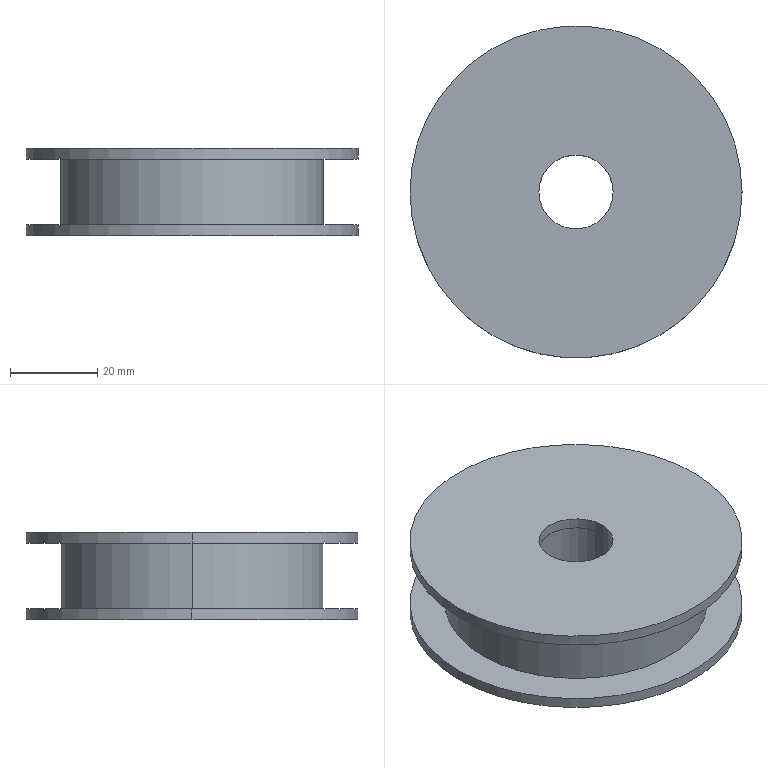Part | STEP file | WHEEL_111V11 | 3 solids | 18 faces | box 76 x 76 x 20 mm | volume 60554 mm3 | cylinder 12 | plane 6 | commonest cylinder face diameters 17 x6 76 x4 60 x2
STEP:
#1=CARTESIAN_POINT('',(0.,0.,0.));
#2=DIRECTION('',(0.,0.,1.));
#3=DIRECTION('',(1.,0.,0.));
#4=AXIS2_PLACEMENT_3D('',#1,#2,#3);
#5=CARTESIAN_POINT('',(-8.5,0.,15.));
#6=VERTEX_POINT('',#5);
#7=CARTESIAN_POINT('',(-8.5,0.,0.));
#8=VERTEX_POINT('',#7);
#9=CARTESIAN_POINT('',(-8.5,0.,15.));
#10=DIRECTION('',(0.,0.,-1.));
#11=VECTOR('',#10,1.);
#12=LINE('',#9,#11);
#13=CARTESIAN_POINT('',(0.,0.,15.));
#14=DIRECTION('',(0.,0.,-1.));
#15=DIRECTION('',(-1.,0.,0.));
#16=AXIS2_PLACEMENT_3D('',#13,#14,#15);
#17=CYLINDRICAL_SURFACE('',#16,8.5);
#18=CARTESIAN_POINT('',(6.283,0.));
#19=DIRECTION('',(0.,1.));
#20=VECTOR('',#19,1.);
#21=LINE('',#18,#20);
#22=(GEOMETRIC_REPRESENTATION_CONTEXT(2)PARAMETRIC_REPRESENTATION_CONTEXT()REPRESENTATION_CONTEXT('',''));
#23=DEFINITIONAL_REPRESENTATION('',(#21),#22);
#24=PCURVE('',#17,#23);
#25=CARTESIAN_POINT('',(0.,0.,15.));
#26=DIRECTION('',(0.,0.,-1.));
#27=DIRECTION('',(-1.,0.,0.));
#28=AXIS2_PLACEMENT_3D('',#25,#26,#27);
#29=CYLINDRICAL_SURFACE('',#28,8.5);
#30=CARTESIAN_POINT('',(0.,0.));
#31=DIRECTION('',(0.,1.));
#32=VECTOR('',#31,1.);
#33=LINE('',#30,#32);
#34=(GEOMETRIC_REPRESENTATION_CONTEXT(2)PARAMETRIC_REPRESENTATION_CONTEXT()REPRESENTATION_CONTEXT('',''));
#35=DEFINITIONAL_REPRESENTATION('',(#33),#34);
#36=PCURVE('',#29,#35);
#37=SURFACE_CURVE('',#12,(#24,#36),.PCURVE_S1.);
#38=EDGE_CURVE('',#6,#8,#37,.T.);
#39=ORIENTED_EDGE('',*,*,#38,.T.);
#40=CARTESIAN_POINT('',(8.5,0.,0.));
#41=VERTEX_POINT('',#40);
#42=CARTESIAN_POINT('',(0.,0.,0.));
#43=DIRECTION('',(0.,0.,1.));
#44=DIRECTION('',(1.,0.,0.));
#45=AXIS2_PLACEMENT_3D('',#42,#43,#44);
#46=CIRCLE('',#45,8.5);
#47=CARTESIAN_POINT('',(9.425,15.));
#48=DIRECTION('',(-1.,0.));
#49=VECTOR('',#48,1.);
#50=LINE('',#47,#49);
#51=(GEOMETRIC_REPRESENTATION_CONTEXT(2)PARAMETRIC_REPRESENTATION_CONTEXT()REPRESENTATION_CONTEXT('',''));
#52=DEFINITIONAL_REPRESENTATION('',(#50),#51);
#53=PCURVE('',#17,#52);
#54=CARTESIAN_POINT('',(0.,0.,0.));
#55=DIRECTION('',(0.,0.,1.));
#56=DIRECTION('',(1.,0.,0.));
#57=AXIS2_PLACEMENT_3D('',#54,#55,#56);
#58=PLANE('',#57);
#59=CARTESIAN_POINT('',(0.,0.));
#60=DIRECTION('',(1.,0.));
#61=AXIS2_PLACEMENT_2D('',#59,#60);
#62=CIRCLE('',#61,8.5);
#63=(GEOMETRIC_REPRESENTATION_CONTEXT(2)PARAMETRIC_REPRESENTATION_CONTEXT()REPRESENTATION_CONTEXT('',''));
#64=DEFINITIONAL_REPRESENTATION('',(#62),#63);
#65=PCURVE('',#58,#64);
#66=SURFACE_CURVE('',#46,(#53,#65),.PCURVE_S1.);
#67=EDGE_CURVE('',#8,#41,#66,.T.);
#68=ORIENTED_EDGE('',*,*,#67,.T.);
#69=CARTESIAN_POINT('',(8.5,0.,15.));
#70=VERTEX_POINT('',#69);
#71=CARTESIAN_POINT('',(8.5,0.,15.));
#72=DIRECTION('',(0.,0.,-1.));
#73=VECTOR('',#72,1.);
#74=LINE('',#71,#73);
#75=CARTESIAN_POINT('',(3.142,0.));
#76=DIRECTION('',(0.,1.));
#77=VECTOR('',#76,1.);
#78=LINE('',#75,#77);
#79=(GEOMETRIC_REPRESENTATION_CONTEXT(2)PARAMETRIC_REPRESENTATION_CONTEXT()REPRESENTATION_CONTEXT('',''));
#80=DEFINITIONAL_REPRESENTATION('',(#78),#79);
#81=PCURVE('',#17,#80);
#82=CARTESIAN_POINT('',(3.142,0.));
#83=DIRECTION('',(0.,1.));
#84=VECTOR('',#83,1.);
#85=LINE('',#82,#84);
#86=(GEOMETRIC_REPRESENTATION_CONTEXT(2)PARAMETRIC_REPRESENTATION_CONTEXT()REPRESENTATION_CONTEXT('',''));
#87=DEFINITIONAL_REPRESENTATION('',(#85),#86);
#88=PCURVE('',#29,#87);
#89=SURFACE_CURVE('',#74,(#81,#88),.PCURVE_S1.);
#90=EDGE_CURVE('',#70,#41,#89,.T.);
#91=ORIENTED_EDGE('',*,*,#90,.F.);
#92=CARTESIAN_POINT('',(0.,0.,15.));
#93=DIRECTION('',(0.,0.,1.));
#94=DIRECTION('',(1.,0.,0.));
#95=AXIS2_PLACEMENT_3D('',#92,#93,#94);
#96=CIRCLE('',#95,8.5);
#97=CARTESIAN_POINT('',(9.425,0.));
#98=DIRECTION('',(-1.,0.));
#99=VECTOR('',#98,1.);
#100=LINE('',#97,#99);
#101=(GEOMETRIC_REPRESENTATION_CONTEXT(2)PARAMETRIC_REPRESENTATION_CONTEXT()REPRESENTATION_CONTEXT('',''));
#102=DEFINITIONAL_REPRESENTATION('',(#100),#101);
#103=PCURVE('',#17,#102);
#104=CARTESIAN_POINT('',(0.,0.,15.));
#105=DIRECTION('',(0.,0.,1.));
#106=DIRECTION('',(1.,0.,0.));
#107=AXIS2_PLACEMENT_3D('',#104,#105,#106);
#108=PLANE('',#107);
#109=CARTESIAN_POINT('',(0.,0.));
#110=DIRECTION('',(1.,0.));
#111=AXIS2_PLACEMENT_2D('',#109,#110);
#112=CIRCLE('',#111,8.5);
#113=(GEOMETRIC_REPRESENTATION_CONTEXT(2)PARAMETRIC_REPRESENTATION_CONTEXT()REPRESENTATION_CONTEXT('',''));
#114=DEFINITIONAL_REPRESENTATION('',(#112),#113);
#115=PCURVE('',#108,#114);
#116=SURFACE_CURVE('',#96,(#103,#115),.PCURVE_S1.);
#117=EDGE_CURVE('',#6,#70,#116,.T.);
#118=ORIENTED_EDGE('',*,*,#117,.F.);
#119=EDGE_LOOP('',(#39,#68,#91,#118));
#120=FACE_BOUND('',#119,.F.);
#121=ADVANCED_FACE('',(#120),#17,.F.);
#122=CARTESIAN_POINT('',(30.,0.,15.));
#123=VERTEX_POINT('',#122);
#124=CARTESIAN_POINT('',(-30.,0.,15.));
#125=VERTEX_POINT('',#124);
#126=CARTESIAN_POINT('',(0.,0.,15.));
#127=DIRECTION('',(0.,0.,1.));
#128=DIRECTION('',(1.,0.,0.));
#129=AXIS2_PLACEMENT_3D('',#126,#127,#128);
#130=CIRCLE('',#129,30.);
#131=CARTESIAN_POINT('',(0.,0.,15.));
#132=DIRECTION('',(0.,0.,-1.));
#133=DIRECTION('',(-1.,0.,0.));
#134=AXIS2_PLACEMENT_3D('',#131,#132,#133);
#135=CYLINDRICAL_SURFACE('',#134,30.);
#136=CARTESIAN_POINT('',(3.142,0.));
#137=DIRECTION('',(-1.,0.));
#138=VECTOR('',#137,1.);
#139=LINE('',#136,#138);
#140=(GEOMETRIC_REPRESENTATION_CONTEXT(2)PARAMETRIC_REPRESENTATION_CONTEXT()REPRESENTATION_CONTEXT('',''));
#141=DEFINITIONAL_REPRESENTATION('',(#139),#140);
#142=PCURVE('',#135,#141);
#143=CARTESIAN_POINT('',(0.,0.));
#144=DIRECTION('',(1.,0.));
#145=AXIS2_PLACEMENT_2D('',#143,#144);
#146=CIRCLE('',#145,30.);
#147=(GEOMETRIC_REPRESENTATION_CONTEXT(2)PARAMETRIC_REPRESENTATION_CONTEXT()REPRESENTATION_CONTEXT('',''));
#148=DEFINITIONAL_REPRESENTATION('',(#146),#147);
#149=PCURVE('',#108,#148);
#150=SURFACE_CURVE('',#130,(#142,#149),.PCURVE_S1.);
#151=EDGE_CURVE('',#123,#125,#150,.T.);
#152=ORIENTED_EDGE('',*,*,#151,.F.);
#153=CARTESIAN_POINT('',(30.,0.,0.));
#154=VERTEX_POINT('',#153);
#155=CARTESIAN_POINT('',(30.,0.,15.));
#156=DIRECTION('',(0.,0.,-1.));
#157=VECTOR('',#156,1.);
#158=LINE('',#155,#157);
#159=CARTESIAN_POINT('',(3.142,0.));
#160=DIRECTION('',(0.,1.));
#161=VECTOR('',#160,1.);
#162=LINE('',#159,#161);
#163=(GEOMETRIC_REPRESENTATION_CONTEXT(2)PARAMETRIC_REPRESENTATION_CONTEXT()REPRESENTATION_CONTEXT('',''));
#164=DEFINITIONAL_REPRESENTATION('',(#162),#163);
#165=PCURVE('',#135,#164);
#166=CARTESIAN_POINT('',(0.,0.,15.));
#167=DIRECTION('',(0.,0.,-1.));
#168=DIRECTION('',(-1.,0.,0.));
#169=AXIS2_PLACEMENT_3D('',#166,#167,#168);
#170=CYLINDRICAL_SURFACE('',#169,30.);
#171=CARTESIAN_POINT('',(3.142,0.));
#172=DIRECTION('',(0.,1.));
#173=VECTOR('',#172,1.);
#174=LINE('',#171,#173);
#175=(GEOMETRIC_REPRESENTATION_CONTEXT(2)PARAMETRIC_REPRESENTATION_CONTEXT()REPRESENTATION_CONTEXT('',''));
#176=DEFINITIONAL_REPRESENTATION('',(#174),#175);
#177=PCURVE('',#170,#176);
#178=SURFACE_CURVE('',#158,(#165,#177),.PCURVE_S1.);
#179=EDGE_CURVE('',#123,#154,#178,.T.);
#180=ORIENTED_EDGE('',*,*,#179,.T.);
#181=CARTESIAN_POINT('',(-30.,0.,0.));
#182=VERTEX_POINT('',#181);
#183=CARTESIAN_POINT('',(0.,0.,0.));
#184=DIRECTION('',(0.,0.,1.));
#185=DIRECTION('',(1.,0.,0.));
#186=AXIS2_PLACEMENT_3D('',#183,#184,#185);
#187=CIRCLE('',#186,30.);
#188=CARTESIAN_POINT('',(3.142,15.));
#189=DIRECTION('',(-1.,0.));
#190=VECTOR('',#189,1.);
#191=LINE('',#188,#190);
#192=(GEOMETRIC_REPRESENTATION_CONTEXT(2)PARAMETRIC_REPRESENTATION_CONTEXT()REPRESENTATION_CONTEXT('',''));
#193=DEFINITIONAL_REPRESENTATION('',(#191),#192);
#194=PCURVE('',#135,#193);
#195=CARTESIAN_POINT('',(0.,0.));
#196=DIRECTION('',(1.,0.));
#197=AXIS2_PLACEMENT_2D('',#195,#196);
#198=CIRCLE('',#197,30.);
#199=(GEOMETRIC_REPRESENTATION_CONTEXT(2)PARAMETRIC_REPRESENTATION_CONTEXT()REPRESENTATION_CONTEXT('',''));
#200=DEFINITIONAL_REPRESENTATION('',(#198),#199);
#201=PCURVE('',#58,#200);
#202=SURFACE_CURVE('',#187,(#194,#201),.PCURVE_S1.);
#203=EDGE_CURVE('',#154,#182,#202,.T.);
#204=ORIENTED_EDGE('',*,*,#203,.T.);
#205=CARTESIAN_POINT('',(-30.,0.,15.));
#206=DIRECTION('',(0.,0.,-1.));
#207=VECTOR('',#206,1.);
#208=LINE('',#205,#207);
#209=CARTESIAN_POINT('',(0.,0.));
#210=DIRECTION('',(0.,1.));
#211=VECTOR('',#210,1.);
#212=LINE('',#209,#211);
#213=(GEOMETRIC_REPRESENTATION_CONTEXT(2)PARAMETRIC_REPRESENTATION_CONTEXT()REPRESENTATION_CONTEXT('',''));
#214=DEFINITIONAL_REPRESENTATION('',(#212),#213);
#215=PCURVE('',#135,#214);
#216=CARTESIAN_POINT('',(6.283,0.));
#217=DIRECTION('',(0.,1.));
#218=VECTOR('',#217,1.);
#219=LINE('',#216,#218);
#220=(GEOMETRIC_REPRESENTATION_CONTEXT(2)PARAMETRIC_REPRESENTATION_CONTEXT()REPRESENTATION_CONTEXT('',''));
#221=DEFINITIONAL_REPRESENTATION('',(#219),#220);
#222=PCURVE('',#170,#221);
#223=SURFACE_CURVE('',#208,(#215,#222),.PCURVE_S1.);
#224=EDGE_CURVE('',#125,#182,#223,.T.);
#225=ORIENTED_EDGE('',*,*,#224,.F.);
#226=EDGE_LOOP('',(#152,#180,#204,#225));
#227=FACE_BOUND('',#226,.T.);
#228=ADVANCED_FACE('',(#227),#135,.T.);
#229=CARTESIAN_POINT('',(0.,0.,15.));
#230=DIRECTION('',(0.,0.,1.));
#231=DIRECTION('',(1.,0.,0.));
#232=AXIS2_PLACEMENT_3D('',#229,#230,#231);
#233=CIRCLE('',#232,30.);
#234=CARTESIAN_POINT('',(0.,0.));
#235=DIRECTION('',(1.,0.));
#236=AXIS2_PLACEMENT_2D('',#234,#235);
#237=CIRCLE('',#236,30.);
#238=(GEOMETRIC_REPRESENTATION_CONTEXT(2)PARAMETRIC_REPRESENTATION_CONTEXT()REPRESENTATION_CONTEXT('',''));
#239=DEFINITIONAL_REPRESENTATION('',(#237),#238);
#240=PCURVE('',#108,#239);
#241=CARTESIAN_POINT('',(9.425,0.));
#242=DIRECTION('',(-1.,0.));
#243=VECTOR('',#242,1.);
#244=LINE('',#241,#243);
#245=(GEOMETRIC_REPRESENTATION_CONTEXT(2)PARAMETRIC_REPRESENTATION_CONTEXT()REPRESENTATION_CONTEXT('',''));
#246=DEFINITIONAL_REPRESENTATION('',(#244),#245);
#247=PCURVE('',#170,#246);
#248=SURFACE_CURVE('',#233,(#240,#247),.PCURVE_S1.);
#249=EDGE_CURVE('',#125,#123,#248,.T.);
#250=ORIENTED_EDGE('',*,*,#249,.T.);
#251=ORIENTED_EDGE('',*,*,#151,.T.);
#252=EDGE_LOOP('',(#250,#251));
#253=FACE_BOUND('',#252,.T.);
#254=ORIENTED_EDGE('',*,*,#117,.F.);
#255=CARTESIAN_POINT('',(0.,0.,15.));
#256=DIRECTION('',(0.,0.,1.));
#257=DIRECTION('',(1.,0.,0.));
#258=AXIS2_PLACEMENT_3D('',#255,#256,#257);
#259=CIRCLE('',#258,8.5);
#260=CARTESIAN_POINT('',(0.,0.));
#261=DIRECTION('',(1.,0.));
#262=AXIS2_PLACEMENT_2D('',#260,#261);
#263=CIRCLE('',#262,8.5);
#264=(GEOMETRIC_REPRESENTATION_CONTEXT(2)PARAMETRIC_REPRESENTATION_CONTEXT()REPRESENTATION_CONTEXT('',''));
#265=DEFINITIONAL_REPRESENTATION('',(#263),#264);
#266=PCURVE('',#108,#265);
#267=CARTESIAN_POINT('',(3.142,0.));
#268=DIRECTION('',(-1.,0.));
#269=VECTOR('',#268,1.);
#270=LINE('',#267,#269);
#271=(GEOMETRIC_REPRESENTATION_CONTEXT(2)PARAMETRIC_REPRESENTATION_CONTEXT()REPRESENTATION_CONTEXT('',''));
#272=DEFINITIONAL_REPRESENTATION('',(#270),#271);
#273=PCURVE('',#29,#272);
#274=SURFACE_CURVE('',#259,(#266,#273),.PCURVE_S1.);
#275=EDGE_CURVE('',#70,#6,#274,.T.);
#276=ORIENTED_EDGE('',*,*,#275,.F.);
#277=EDGE_LOOP('',(#254,#276));
#278=FACE_BOUND('',#277,.T.);
#279=ADVANCED_FACE('',(#253,#278),#108,.T.);
#280=CARTESIAN_POINT('',(0.,0.,0.));
#281=DIRECTION('',(0.,0.,1.));
#282=DIRECTION('',(1.,0.,0.));
#283=AXIS2_PLACEMENT_3D('',#280,#281,#282);
#284=CIRCLE('',#283,30.);
#285=CARTESIAN_POINT('',(0.,0.));
#286=DIRECTION('',(1.,0.));
#287=AXIS2_PLACEMENT_2D('',#285,#286);
#288=CIRCLE('',#287,30.);
#289=(GEOMETRIC_REPRESENTATION_CONTEXT(2)PARAMETRIC_REPRESENTATION_CONTEXT()REPRESENTATION_CONTEXT('',''));
#290=DEFINITIONAL_REPRESENTATION('',(#288),#289);
#291=PCURVE('',#58,#290);
#292=CARTESIAN_POINT('',(9.425,15.));
#293=DIRECTION('',(-1.,0.));
#294=VECTOR('',#293,1.);
#295=LINE('',#292,#294);
#296=(GEOMETRIC_REPRESENTATION_CONTEXT(2)PARAMETRIC_REPRESENTATION_CONTEXT()REPRESENTATION_CONTEXT('',''));
#297=DEFINITIONAL_REPRESENTATION('',(#295),#296);
#298=PCURVE('',#170,#297);
#299=SURFACE_CURVE('',#284,(#291,#298),.PCURVE_S1.);
#300=EDGE_CURVE('',#182,#154,#299,.T.);
#301=ORIENTED_EDGE('',*,*,#300,.F.);
#302=ORIENTED_EDGE('',*,*,#203,.F.);
#303=EDGE_LOOP('',(#301,#302));
#304=FACE_BOUND('',#303,.T.);
#305=ORIENTED_EDGE('',*,*,#67,.T.);
#306=CARTESIAN_POINT('',(0.,0.,0.));
#307=DIRECTION('',(0.,0.,1.));
#308=DIRECTION('',(1.,0.,0.));
#309=AXIS2_PLACEMENT_3D('',#306,#307,#308);
#310=CIRCLE('',#309,8.5);
#311=CARTESIAN_POINT('',(0.,0.));
#312=DIRECTION('',(1.,0.));
#313=AXIS2_PLACEMENT_2D('',#311,#312);
#314=CIRCLE('',#313,8.5);
#315=(GEOMETRIC_REPRESENTATION_CONTEXT(2)PARAMETRIC_REPRESENTATION_CONTEXT()REPRESENTATION_CONTEXT('',''));
#316=DEFINITIONAL_REPRESENTATION('',(#314),#315);
#317=PCURVE('',#58,#316);
#318=CARTESIAN_POINT('',(3.142,15.));
#319=DIRECTION('',(-1.,0.));
#320=VECTOR('',#319,1.);
#321=LINE('',#318,#320);
#322=(GEOMETRIC_REPRESENTATION_CONTEXT(2)PARAMETRIC_REPRESENTATION_CONTEXT()REPRESENTATION_CONTEXT('',''));
#323=DEFINITIONAL_REPRESENTATION('',(#321),#322);
#324=PCURVE('',#29,#323);
#325=SURFACE_CURVE('',#310,(#317,#324),.PCURVE_S1.);
#326=EDGE_CURVE('',#41,#8,#325,.T.);
#327=ORIENTED_EDGE('',*,*,#326,.T.);
#328=EDGE_LOOP('',(#305,#327));
#329=FACE_BOUND('',#328,.T.);
#330=ADVANCED_FACE('',(#304,#329),#58,.F.);
#331=ORIENTED_EDGE('',*,*,#179,.F.);
#332=ORIENTED_EDGE('',*,*,#249,.F.);
#333=ORIENTED_EDGE('',*,*,#224,.T.);
#334=ORIENTED_EDGE('',*,*,#300,.T.);
#335=EDGE_LOOP('',(#331,#332,#333,#334));
#336=FACE_BOUND('',#335,.T.);
#337=ADVANCED_FACE('',(#336),#170,.T.);
#338=ORIENTED_EDGE('',*,*,#326,.T.);
#339=ORIENTED_EDGE('',*,*,#38,.F.);
#340=ORIENTED_EDGE('',*,*,#275,.F.);
#341=ORIENTED_EDGE('',*,*,#90,.T.);
#342=EDGE_LOOP('',(#338,#339,#340,#341));
#343=FACE_BOUND('',#342,.F.);
#344=ADVANCED_FACE('',(#343),#29,.F.);
#345=CLOSED_SHELL('',(#121,#228,#279,#330,#337,#344));
#346=MANIFOLD_SOLID_BREP('',#345);
#347=CARTESIAN_POINT('',(-8.5,0.,17.5));
#348=VERTEX_POINT('',#347);
#349=CARTESIAN_POINT('',(-8.5,0.,15.));
#350=VERTEX_POINT('',#349);
#351=CARTESIAN_POINT('',(-8.5,0.,17.5));
#352=DIRECTION('',(0.,0.,-1.));
#353=VECTOR('',#352,1.);
#354=LINE('',#351,#353);
#355=CARTESIAN_POINT('',(0.,0.,17.5));
#356=DIRECTION('',(0.,0.,-1.));
#357=DIRECTION('',(-1.,0.,0.));
#358=AXIS2_PLACEMENT_3D('',#355,#356,#357);
#359=CYLINDRICAL_SURFACE('',#358,8.5);
#360=CARTESIAN_POINT('',(6.283,0.));
#361=DIRECTION('',(0.,1.));
#362=VECTOR('',#361,1.);
#363=LINE('',#360,#362);
#364=(GEOMETRIC_REPRESENTATION_CONTEXT(2)PARAMETRIC_REPRESENTATION_CONTEXT()REPRESENTATION_CONTEXT('',''));
#365=DEFINITIONAL_REPRESENTATION('',(#363),#364);
#366=PCURVE('',#359,#365);
#367=CARTESIAN_POINT('',(0.,0.,17.5));
#368=DIRECTION('',(0.,0.,-1.));
#369=DIRECTION('',(-1.,0.,0.));
#370=AXIS2_PLACEMENT_3D('',#367,#368,#369);
#371=CYLINDRICAL_SURFACE('',#370,8.5);
#372=CARTESIAN_POINT('',(0.,0.));
#373=DIRECTION('',(0.,1.));
#374=VECTOR('',#373,1.);
#375=LINE('',#372,#374);
#376=(GEOMETRIC_REPRESENTATION_CONTEXT(2)PARAMETRIC_REPRESENTATION_CONTEXT()REPRESENTATION_CONTEXT('',''));
#377=DEFINITIONAL_REPRESENTATION('',(#375),#376);
#378=PCURVE('',#371,#377);
#379=SURFACE_CURVE('',#354,(#366,#378),.PCURVE_S1.);
#380=EDGE_CURVE('',#348,#350,#379,.T.);
#381=ORIENTED_EDGE('',*,*,#380,.T.);
#382=CARTESIAN_POINT('',(8.5,0.,15.));
#383=VERTEX_POINT('',#382);
#384=CARTESIAN_POINT('',(0.,0.,15.));
#385=DIRECTION('',(0.,0.,1.));
#386=DIRECTION('',(1.,0.,0.));
#387=AXIS2_PLACEMENT_3D('',#384,#385,#386);
#388=CIRCLE('',#387,8.5);
#389=CARTESIAN_POINT('',(9.425,2.5));
#390=DIRECTION('',(-1.,0.));
#391=VECTOR('',#390,1.);
#392=LINE('',#389,#391);
#393=(GEOMETRIC_REPRESENTATION_CONTEXT(2)PARAMETRIC_REPRESENTATION_CONTEXT()REPRESENTATION_CONTEXT('',''));
#394=DEFINITIONAL_REPRESENTATION('',(#392),#393);
#395=PCURVE('',#359,#394);
#396=CARTESIAN_POINT('',(0.,0.,15.));
#397=DIRECTION('',(0.,0.,1.));
#398=DIRECTION('',(1.,0.,0.));
#399=AXIS2_PLACEMENT_3D('',#396,#397,#398);
#400=PLANE('',#399);
#401=CARTESIAN_POINT('',(0.,0.));
#402=DIRECTION('',(1.,0.));
#403=AXIS2_PLACEMENT_2D('',#401,#402);
#404=CIRCLE('',#403,8.5);
#405=(GEOMETRIC_REPRESENTATION_CONTEXT(2)PARAMETRIC_REPRESENTATION_CONTEXT()REPRESENTATION_CONTEXT('',''));
#406=DEFINITIONAL_REPRESENTATION('',(#404),#405);
#407=PCURVE('',#400,#406);
#408=SURFACE_CURVE('',#388,(#395,#407),.PCURVE_S1.);
#409=EDGE_CURVE('',#350,#383,#408,.T.);
#410=ORIENTED_EDGE('',*,*,#409,.T.);
#411=CARTESIAN_POINT('',(8.5,0.,17.5));
#412=VERTEX_POINT('',#411);
#413=CARTESIAN_POINT('',(8.5,0.,17.5));
#414=DIRECTION('',(0.,0.,-1.));
#415=VECTOR('',#414,1.);
#416=LINE('',#413,#415);
#417=CARTESIAN_POINT('',(3.142,0.));
#418=DIRECTION('',(0.,1.));
#419=VECTOR('',#418,1.);
#420=LINE('',#417,#419);
#421=(GEOMETRIC_REPRESENTATION_CONTEXT(2)PARAMETRIC_REPRESENTATION_CONTEXT()REPRESENTATION_CONTEXT('',''));
#422=DEFINITIONAL_REPRESENTATION('',(#420),#421);
#423=PCURVE('',#359,#422);
#424=CARTESIAN_POINT('',(3.142,0.));
#425=DIRECTION('',(0.,1.));
#426=VECTOR('',#425,1.);
#427=LINE('',#424,#426);
#428=(GEOMETRIC_REPRESENTATION_CONTEXT(2)PARAMETRIC_REPRESENTATION_CONTEXT()REPRESENTATION_CONTEXT('',''));
#429=DEFINITIONAL_REPRESENTATION('',(#427),#428);
#430=PCURVE('',#371,#429);
#431=SURFACE_CURVE('',#416,(#423,#430),.PCURVE_S1.);
#432=EDGE_CURVE('',#412,#383,#431,.T.);
#433=ORIENTED_EDGE('',*,*,#432,.F.);
#434=CARTESIAN_POINT('',(0.,0.,17.5));
#435=DIRECTION('',(0.,0.,1.));
#436=DIRECTION('',(1.,0.,0.));
#437=AXIS2_PLACEMENT_3D('',#434,#435,#436);
#438=CIRCLE('',#437,8.5);
#439=CARTESIAN_POINT('',(9.425,0.));
#440=DIRECTION('',(-1.,0.));
#441=VECTOR('',#440,1.);
#442=LINE('',#439,#441);
#443=(GEOMETRIC_REPRESENTATION_CONTEXT(2)PARAMETRIC_REPRESENTATION_CONTEXT()REPRESENTATION_CONTEXT('',''));
#444=DEFINITIONAL_REPRESENTATION('',(#442),#443);
#445=PCURVE('',#359,#444);
#446=CARTESIAN_POINT('',(0.,0.,17.5));
#447=DIRECTION('',(0.,0.,1.));
#448=DIRECTION('',(1.,0.,0.));
#449=AXIS2_PLACEMENT_3D('',#446,#447,#448);
#450=PLANE('',#449);
#451=CARTESIAN_POINT('',(0.,0.));
#452=DIRECTION('',(1.,0.));
#453=AXIS2_PLACEMENT_2D('',#451,#452);
#454=CIRCLE('',#453,8.5);
#455=(GEOMETRIC_REPRESENTATION_CONTEXT(2)PARAMETRIC_REPRESENTATION_CONTEXT()REPRESENTATION_CONTEXT('',''));
#456=DEFINITIONAL_REPRESENTATION('',(#454),#455);
#457=PCURVE('',#450,#456);
#458=SURFACE_CURVE('',#438,(#445,#457),.PCURVE_S1.);
#459=EDGE_CURVE('',#348,#412,#458,.T.);
#460=ORIENTED_EDGE('',*,*,#459,.F.);
#461=EDGE_LOOP('',(#381,#410,#433,#460));
#462=FACE_BOUND('',#461,.F.);
#463=ADVANCED_FACE('',(#462),#359,.F.);
#464=CARTESIAN_POINT('',(38.,0.,17.5));
#465=VERTEX_POINT('',#464);
#466=CARTESIAN_POINT('',(-38.,0.,17.5));
#467=VERTEX_POINT('',#466);
#468=CARTESIAN_POINT('',(0.,0.,17.5));
#469=DIRECTION('',(0.,0.,1.));
#470=DIRECTION('',(1.,0.,0.));
#471=AXIS2_PLACEMENT_3D('',#468,#469,#470);
#472=CIRCLE('',#471,38.);
#473=CARTESIAN_POINT('',(0.,0.,17.5));
#474=DIRECTION('',(0.,0.,-1.));
#475=DIRECTION('',(-1.,0.,0.));
#476=AXIS2_PLACEMENT_3D('',#473,#474,#475);
#477=CYLINDRICAL_SURFACE('',#476,38.);
#478=CARTESIAN_POINT('',(3.142,0.));
#479=DIRECTION('',(-1.,0.));
#480=VECTOR('',#479,1.);
#481=LINE('',#478,#480);
#482=(GEOMETRIC_REPRESENTATION_CONTEXT(2)PARAMETRIC_REPRESENTATION_CONTEXT()REPRESENTATION_CONTEXT('',''));
#483=DEFINITIONAL_REPRESENTATION('',(#481),#482);
#484=PCURVE('',#477,#483);
#485=CARTESIAN_POINT('',(0.,0.));
#486=DIRECTION('',(1.,0.));
#487=AXIS2_PLACEMENT_2D('',#485,#486);
#488=CIRCLE('',#487,38.);
#489=(GEOMETRIC_REPRESENTATION_CONTEXT(2)PARAMETRIC_REPRESENTATION_CONTEXT()REPRESENTATION_CONTEXT('',''));
#490=DEFINITIONAL_REPRESENTATION('',(#488),#489);
#491=PCURVE('',#450,#490);
#492=SURFACE_CURVE('',#472,(#484,#491),.PCURVE_S1.);
#493=EDGE_CURVE('',#465,#467,#492,.T.);
#494=ORIENTED_EDGE('',*,*,#493,.F.);
#495=CARTESIAN_POINT('',(38.,0.,15.));
#496=VERTEX_POINT('',#495);
#497=CARTESIAN_POINT('',(38.,0.,17.5));
#498=DIRECTION('',(0.,0.,-1.));
#499=VECTOR('',#498,1.);
#500=LINE('',#497,#499);
#501=CARTESIAN_POINT('',(3.142,0.));
#502=DIRECTION('',(0.,1.));
#503=VECTOR('',#502,1.);
#504=LINE('',#501,#503);
#505=(GEOMETRIC_REPRESENTATION_CONTEXT(2)PARAMETRIC_REPRESENTATION_CONTEXT()REPRESENTATION_CONTEXT('',''));
#506=DEFINITIONAL_REPRESENTATION('',(#504),#505);
#507=PCURVE('',#477,#506);
#508=CARTESIAN_POINT('',(0.,0.,17.5));
#509=DIRECTION('',(0.,0.,-1.));
#510=DIRECTION('',(-1.,0.,0.));
#511=AXIS2_PLACEMENT_3D('',#508,#509,#510);
#512=CYLINDRICAL_SURFACE('',#511,38.);
#513=CARTESIAN_POINT('',(3.142,0.));
#514=DIRECTION('',(0.,1.));
#515=VECTOR('',#514,1.);
#516=LINE('',#513,#515);
#517=(GEOMETRIC_REPRESENTATION_CONTEXT(2)PARAMETRIC_REPRESENTATION_CONTEXT()REPRESENTATION_CONTEXT('',''));
#518=DEFINITIONAL_REPRESENTATION('',(#516),#517);
#519=PCURVE('',#512,#518);
#520=SURFACE_CURVE('',#500,(#507,#519),.PCURVE_S1.);
#521=EDGE_CURVE('',#465,#496,#520,.T.);
#522=ORIENTED_EDGE('',*,*,#521,.T.);
#523=CARTESIAN_POINT('',(-38.,0.,15.));
#524=VERTEX_POINT('',#523);
#525=CARTESIAN_POINT('',(0.,0.,15.));
#526=DIRECTION('',(0.,0.,1.));
#527=DIRECTION('',(1.,0.,0.));
#528=AXIS2_PLACEMENT_3D('',#525,#526,#527);
#529=CIRCLE('',#528,38.);
#530=CARTESIAN_POINT('',(3.142,2.5));
#531=DIRECTION('',(-1.,0.));
#532=VECTOR('',#531,1.);
#533=LINE('',#530,#532);
#534=(GEOMETRIC_REPRESENTATION_CONTEXT(2)PARAMETRIC_REPRESENTATION_CONTEXT()REPRESENTATION_CONTEXT('',''));
#535=DEFINITIONAL_REPRESENTATION('',(#533),#534);
#536=PCURVE('',#477,#535);
#537=CARTESIAN_POINT('',(0.,0.));
#538=DIRECTION('',(1.,0.));
#539=AXIS2_PLACEMENT_2D('',#537,#538);
#540=CIRCLE('',#539,38.);
#541=(GEOMETRIC_REPRESENTATION_CONTEXT(2)PARAMETRIC_REPRESENTATION_CONTEXT()REPRESENTATION_CONTEXT('',''));
#542=DEFINITIONAL_REPRESENTATION('',(#540),#541);
#543=PCURVE('',#400,#542);
#544=SURFACE_CURVE('',#529,(#536,#543),.PCURVE_S1.);
#545=EDGE_CURVE('',#496,#524,#544,.T.);
#546=ORIENTED_EDGE('',*,*,#545,.T.);
#547=CARTESIAN_POINT('',(-38.,0.,17.5));
#548=DIRECTION('',(0.,0.,-1.));
#549=VECTOR('',#548,1.);
#550=LINE('',#547,#549);
#551=CARTESIAN_POINT('',(0.,0.));
#552=DIRECTION('',(0.,1.));
#553=VECTOR('',#552,1.);
#554=LINE('',#551,#553);
#555=(GEOMETRIC_REPRESENTATION_CONTEXT(2)PARAMETRIC_REPRESENTATION_CONTEXT()REPRESENTATION_CONTEXT('',''));
#556=DEFINITIONAL_REPRESENTATION('',(#554),#555);
#557=PCURVE('',#477,#556);
#558=CARTESIAN_POINT('',(6.283,0.));
#559=DIRECTION('',(0.,1.));
#560=VECTOR('',#559,1.);
#561=LINE('',#558,#560);
#562=(GEOMETRIC_REPRESENTATION_CONTEXT(2)PARAMETRIC_REPRESENTATION_CONTEXT()REPRESENTATION_CONTEXT('',''));
#563=DEFINITIONAL_REPRESENTATION('',(#561),#562);
#564=PCURVE('',#512,#563);
#565=SURFACE_CURVE('',#550,(#557,#564),.PCURVE_S1.);
#566=EDGE_CURVE('',#467,#524,#565,.T.);
#567=ORIENTED_EDGE('',*,*,#566,.F.);
#568=EDGE_LOOP('',(#494,#522,#546,#567));
#569=FACE_BOUND('',#568,.T.);
#570=ADVANCED_FACE('',(#569),#477,.T.);
#571=CARTESIAN_POINT('',(0.,0.,17.5));
#572=DIRECTION('',(0.,0.,1.));
#573=DIRECTION('',(1.,0.,0.));
#574=AXIS2_PLACEMENT_3D('',#571,#572,#573);
#575=CIRCLE('',#574,38.);
#576=CARTESIAN_POINT('',(0.,0.));
#577=DIRECTION('',(1.,0.));
#578=AXIS2_PLACEMENT_2D('',#576,#577);
#579=CIRCLE('',#578,38.);
#580=(GEOMETRIC_REPRESENTATION_CONTEXT(2)PARAMETRIC_REPRESENTATION_CONTEXT()REPRESENTATION_CONTEXT('',''));
#581=DEFINITIONAL_REPRESENTATION('',(#579),#580);
#582=PCURVE('',#450,#581);
#583=CARTESIAN_POINT('',(9.425,0.));
#584=DIRECTION('',(-1.,0.));
#585=VECTOR('',#584,1.);
#586=LINE('',#583,#585);
#587=(GEOMETRIC_REPRESENTATION_CONTEXT(2)PARAMETRIC_REPRESENTATION_CONTEXT()REPRESENTATION_CONTEXT('',''));
#588=DEFINITIONAL_REPRESENTATION('',(#586),#587);
#589=PCURVE('',#512,#588);
#590=SURFACE_CURVE('',#575,(#582,#589),.PCURVE_S1.);
#591=EDGE_CURVE('',#467,#465,#590,.T.);
#592=ORIENTED_EDGE('',*,*,#591,.T.);
#593=ORIENTED_EDGE('',*,*,#493,.T.);
#594=EDGE_LOOP('',(#592,#593));
#595=FACE_BOUND('',#594,.T.);
#596=ORIENTED_EDGE('',*,*,#459,.F.);
#597=CARTESIAN_POINT('',(0.,0.,17.5));
#598=DIRECTION('',(0.,0.,1.));
#599=DIRECTION('',(1.,0.,0.));
#600=AXIS2_PLACEMENT_3D('',#597,#598,#599);
#601=CIRCLE('',#600,8.5);
#602=CARTESIAN_POINT('',(0.,0.));
#603=DIRECTION('',(1.,0.));
#604=AXIS2_PLACEMENT_2D('',#602,#603);
#605=CIRCLE('',#604,8.5);
#606=(GEOMETRIC_REPRESENTATION_CONTEXT(2)PARAMETRIC_REPRESENTATION_CONTEXT()REPRESENTATION_CONTEXT('',''));
#607=DEFINITIONAL_REPRESENTATION('',(#605),#606);
#608=PCURVE('',#450,#607);
#609=CARTESIAN_POINT('',(3.142,0.));
#610=DIRECTION('',(-1.,0.));
#611=VECTOR('',#610,1.);
#612=LINE('',#609,#611);
#613=(GEOMETRIC_REPRESENTATION_CONTEXT(2)PARAMETRIC_REPRESENTATION_CONTEXT()REPRESENTATION_CONTEXT('',''));
#614=DEFINITIONAL_REPRESENTATION('',(#612),#613);
#615=PCURVE('',#371,#614);
#616=SURFACE_CURVE('',#601,(#608,#615),.PCURVE_S1.);
#617=EDGE_CURVE('',#412,#348,#616,.T.);
#618=ORIENTED_EDGE('',*,*,#617,.F.);
#619=EDGE_LOOP('',(#596,#618));
#620=FACE_BOUND('',#619,.T.);
#621=ADVANCED_FACE('',(#595,#620),#450,.T.);
#622=CARTESIAN_POINT('',(0.,0.,15.));
#623=DIRECTION('',(0.,0.,1.));
#624=DIRECTION('',(1.,0.,0.));
#625=AXIS2_PLACEMENT_3D('',#622,#623,#624);
#626=CIRCLE('',#625,38.);
#627=CARTESIAN_POINT('',(0.,0.));
#628=DIRECTION('',(1.,0.));
#629=AXIS2_PLACEMENT_2D('',#627,#628);
#630=CIRCLE('',#629,38.);
#631=(GEOMETRIC_REPRESENTATION_CONTEXT(2)PARAMETRIC_REPRESENTATION_CONTEXT()REPRESENTATION_CONTEXT('',''));
#632=DEFINITIONAL_REPRESENTATION('',(#630),#631);
#633=PCURVE('',#400,#632);
#634=CARTESIAN_POINT('',(9.425,2.5));
#635=DIRECTION('',(-1.,0.));
#636=VECTOR('',#635,1.);
#637=LINE('',#634,#636);
#638=(GEOMETRIC_REPRESENTATION_CONTEXT(2)PARAMETRIC_REPRESENTATION_CONTEXT()REPRESENTATION_CONTEXT('',''));
#639=DEFINITIONAL_REPRESENTATION('',(#637),#638);
#640=PCURVE('',#512,#639);
#641=SURFACE_CURVE('',#626,(#633,#640),.PCURVE_S1.);
#642=EDGE_CURVE('',#524,#496,#641,.T.);
#643=ORIENTED_EDGE('',*,*,#642,.F.);
#644=ORIENTED_EDGE('',*,*,#545,.F.);
#645=EDGE_LOOP('',(#643,#644));
#646=FACE_BOUND('',#645,.T.);
#647=ORIENTED_EDGE('',*,*,#409,.T.);
#648=CARTESIAN_POINT('',(0.,0.,15.));
#649=DIRECTION('',(0.,0.,1.));
#650=DIRECTION('',(1.,0.,0.));
#651=AXIS2_PLACEMENT_3D('',#648,#649,#650);
#652=CIRCLE('',#651,8.5);
#653=CARTESIAN_POINT('',(0.,0.));
#654=DIRECTION('',(1.,0.));
#655=AXIS2_PLACEMENT_2D('',#653,#654);
#656=CIRCLE('',#655,8.5);
#657=(GEOMETRIC_REPRESENTATION_CONTEXT(2)PARAMETRIC_REPRESENTATION_CONTEXT()REPRESENTATION_CONTEXT('',''));
#658=DEFINITIONAL_REPRESENTATION('',(#656),#657);
#659=PCURVE('',#400,#658);
#660=CARTESIAN_POINT('',(3.142,2.5));
#661=DIRECTION('',(-1.,0.));
#662=VECTOR('',#661,1.);
#663=LINE('',#660,#662);
#664=(GEOMETRIC_REPRESENTATION_CONTEXT(2)PARAMETRIC_REPRESENTATION_CONTEXT()REPRESENTATION_CONTEXT('',''));
#665=DEFINITIONAL_REPRESENTATION('',(#663),#664);
#666=PCURVE('',#371,#665);
#667=SURFACE_CURVE('',#652,(#659,#666),.PCURVE_S1.);
#668=EDGE_CURVE('',#383,#350,#667,.T.);
#669=ORIENTED_EDGE('',*,*,#668,.T.);
#670=EDGE_LOOP('',(#647,#669));
#671=FACE_BOUND('',#670,.T.);
#672=ADVANCED_FACE('',(#646,#671),#400,.F.);
#673=ORIENTED_EDGE('',*,*,#521,.F.);
#674=ORIENTED_EDGE('',*,*,#591,.F.);
#675=ORIENTED_EDGE('',*,*,#566,.T.);
#676=ORIENTED_EDGE('',*,*,#642,.T.);
#677=EDGE_LOOP('',(#673,#674,#675,#676));
#678=FACE_BOUND('',#677,.T.);
#679=ADVANCED_FACE('',(#678),#512,.T.);
#680=ORIENTED_EDGE('',*,*,#668,.T.);
#681=ORIENTED_EDGE('',*,*,#380,.F.);
#682=ORIENTED_EDGE('',*,*,#617,.F.);
#683=ORIENTED_EDGE('',*,*,#432,.T.);
#684=EDGE_LOOP('',(#680,#681,#682,#683));
#685=FACE_BOUND('',#684,.F.);
#686=ADVANCED_FACE('',(#685),#371,.F.);
#687=CLOSED_SHELL('',(#463,#570,#621,#672,#679,#686));
#688=MANIFOLD_SOLID_BREP('',#687);
#689=CARTESIAN_POINT('',(8.5,0.,-2.5));
#690=VERTEX_POINT('',#689);
#691=CARTESIAN_POINT('',(8.5,0.,0.));
#692=VERTEX_POINT('',#691);
#693=CARTESIAN_POINT('',(8.5,0.,-2.5));
#694=DIRECTION('',(0.,0.,1.));
#695=VECTOR('',#694,1.);
#696=LINE('',#693,#695);
#697=CARTESIAN_POINT('',(0.,0.,-2.5));
#698=DIRECTION('',(0.,0.,1.));
#699=DIRECTION('',(1.,0.,0.));
#700=AXIS2_PLACEMENT_3D('',#697,#698,#699);
#701=CYLINDRICAL_SURFACE('',#700,8.5);
#702=CARTESIAN_POINT('',(6.283,0.));
#703=DIRECTION('',(0.,1.));
#704=VECTOR('',#703,1.);
#705=LINE('',#702,#704);
#706=(GEOMETRIC_REPRESENTATION_CONTEXT(2)PARAMETRIC_REPRESENTATION_CONTEXT()REPRESENTATION_CONTEXT('',''));
#707=DEFINITIONAL_REPRESENTATION('',(#705),#706);
#708=PCURVE('',#701,#707);
#709=CARTESIAN_POINT('',(0.,0.,-2.5));
#710=DIRECTION('',(0.,0.,1.));
#711=DIRECTION('',(1.,0.,0.));
#712=AXIS2_PLACEMENT_3D('',#709,#710,#711);
#713=CYLINDRICAL_SURFACE('',#712,8.5);
#714=CARTESIAN_POINT('',(0.,0.));
#715=DIRECTION('',(0.,1.));
#716=VECTOR('',#715,1.);
#717=LINE('',#714,#716);
#718=(GEOMETRIC_REPRESENTATION_CONTEXT(2)PARAMETRIC_REPRESENTATION_CONTEXT()REPRESENTATION_CONTEXT('',''));
#719=DEFINITIONAL_REPRESENTATION('',(#717),#718);
#720=PCURVE('',#713,#719);
#721=SURFACE_CURVE('',#696,(#708,#720),.PCURVE_S1.);
#722=EDGE_CURVE('',#690,#692,#721,.T.);
#723=ORIENTED_EDGE('',*,*,#722,.T.);
#724=CARTESIAN_POINT('',(-8.5,0.,0.));
#725=VERTEX_POINT('',#724);
#726=CARTESIAN_POINT('',(0.,0.,0.));
#727=DIRECTION('',(0.,0.,-1.));
#728=DIRECTION('',(-1.,0.,0.));
#729=AXIS2_PLACEMENT_3D('',#726,#727,#728);
#730=CIRCLE('',#729,8.5);
#731=CARTESIAN_POINT('',(9.425,2.5));
#732=DIRECTION('',(-1.,0.));
#733=VECTOR('',#732,1.);
#734=LINE('',#731,#733);
#735=(GEOMETRIC_REPRESENTATION_CONTEXT(2)PARAMETRIC_REPRESENTATION_CONTEXT()REPRESENTATION_CONTEXT('',''));
#736=DEFINITIONAL_REPRESENTATION('',(#734),#735);
#737=PCURVE('',#701,#736);
#738=CARTESIAN_POINT('',(0.,0.,0.));
#739=DIRECTION('',(0.,0.,-1.));
#740=DIRECTION('',(-1.,0.,0.));
#741=AXIS2_PLACEMENT_3D('',#738,#739,#740);
#742=PLANE('',#741);
#743=CARTESIAN_POINT('',(0.,0.));
#744=DIRECTION('',(1.,0.));
#745=AXIS2_PLACEMENT_2D('',#743,#744);
#746=CIRCLE('',#745,8.5);
#747=(GEOMETRIC_REPRESENTATION_CONTEXT(2)PARAMETRIC_REPRESENTATION_CONTEXT()REPRESENTATION_CONTEXT('',''));
#748=DEFINITIONAL_REPRESENTATION('',(#746),#747);
#749=PCURVE('',#742,#748);
#750=SURFACE_CURVE('',#730,(#737,#749),.PCURVE_S1.);
#751=EDGE_CURVE('',#692,#725,#750,.T.);
#752=ORIENTED_EDGE('',*,*,#751,.T.);
#753=CARTESIAN_POINT('',(-8.5,0.,-2.5));
#754=VERTEX_POINT('',#753);
#755=CARTESIAN_POINT('',(-8.5,0.,-2.5));
#756=DIRECTION('',(0.,0.,1.));
#757=VECTOR('',#756,1.);
#758=LINE('',#755,#757);
#759=CARTESIAN_POINT('',(3.142,0.));
#760=DIRECTION('',(0.,1.));
#761=VECTOR('',#760,1.);
#762=LINE('',#759,#761);
#763=(GEOMETRIC_REPRESENTATION_CONTEXT(2)PARAMETRIC_REPRESENTATION_CONTEXT()REPRESENTATION_CONTEXT('',''));
#764=DEFINITIONAL_REPRESENTATION('',(#762),#763);
#765=PCURVE('',#701,#764);
#766=CARTESIAN_POINT('',(3.142,0.));
#767=DIRECTION('',(0.,1.));
#768=VECTOR('',#767,1.);
#769=LINE('',#766,#768);
#770=(GEOMETRIC_REPRESENTATION_CONTEXT(2)PARAMETRIC_REPRESENTATION_CONTEXT()REPRESENTATION_CONTEXT('',''));
#771=DEFINITIONAL_REPRESENTATION('',(#769),#770);
#772=PCURVE('',#713,#771);
#773=SURFACE_CURVE('',#758,(#765,#772),.PCURVE_S1.);
#774=EDGE_CURVE('',#754,#725,#773,.T.);
#775=ORIENTED_EDGE('',*,*,#774,.F.);
#776=CARTESIAN_POINT('',(0.,0.,-2.5));
#777=DIRECTION('',(0.,0.,-1.));
#778=DIRECTION('',(-1.,0.,0.));
#779=AXIS2_PLACEMENT_3D('',#776,#777,#778);
#780=CIRCLE('',#779,8.5);
#781=CARTESIAN_POINT('',(9.425,0.));
#782=DIRECTION('',(-1.,0.));
#783=VECTOR('',#782,1.);
#784=LINE('',#781,#783);
#785=(GEOMETRIC_REPRESENTATION_CONTEXT(2)PARAMETRIC_REPRESENTATION_CONTEXT()REPRESENTATION_CONTEXT('',''));
#786=DEFINITIONAL_REPRESENTATION('',(#784),#785);
#787=PCURVE('',#701,#786);
#788=CARTESIAN_POINT('',(0.,0.,-2.5));
#789=DIRECTION('',(0.,0.,-1.));
#790=DIRECTION('',(-1.,0.,0.));
#791=AXIS2_PLACEMENT_3D('',#788,#789,#790);
#792=PLANE('',#791);
#793=CARTESIAN_POINT('',(0.,0.));
#794=DIRECTION('',(1.,0.));
#795=AXIS2_PLACEMENT_2D('',#793,#794);
#796=CIRCLE('',#795,8.5);
#797=(GEOMETRIC_REPRESENTATION_CONTEXT(2)PARAMETRIC_REPRESENTATION_CONTEXT()REPRESENTATION_CONTEXT('',''));
#798=DEFINITIONAL_REPRESENTATION('',(#796),#797);
#799=PCURVE('',#792,#798);
#800=SURFACE_CURVE('',#780,(#787,#799),.PCURVE_S1.);
#801=EDGE_CURVE('',#690,#754,#800,.T.);
#802=ORIENTED_EDGE('',*,*,#801,.F.);
#803=EDGE_LOOP('',(#723,#752,#775,#802));
#804=FACE_BOUND('',#803,.F.);
#805=ADVANCED_FACE('',(#804),#701,.F.);
#806=CARTESIAN_POINT('',(-38.,0.,-2.5));
#807=VERTEX_POINT('',#806);
#808=CARTESIAN_POINT('',(38.,0.,-2.5));
#809=VERTEX_POINT('',#808);
#810=CARTESIAN_POINT('',(0.,0.,-2.5));
#811=DIRECTION('',(0.,0.,-1.));
#812=DIRECTION('',(-1.,0.,0.));
#813=AXIS2_PLACEMENT_3D('',#810,#811,#812);
#814=CIRCLE('',#813,38.);
#815=CARTESIAN_POINT('',(0.,0.,-2.5));
#816=DIRECTION('',(0.,0.,1.));
#817=DIRECTION('',(1.,0.,0.));
#818=AXIS2_PLACEMENT_3D('',#815,#816,#817);
#819=CYLINDRICAL_SURFACE('',#818,38.);
#820=CARTESIAN_POINT('',(3.142,0.));
#821=DIRECTION('',(-1.,0.));
#822=VECTOR('',#821,1.);
#823=LINE('',#820,#822);
#824=(GEOMETRIC_REPRESENTATION_CONTEXT(2)PARAMETRIC_REPRESENTATION_CONTEXT()REPRESENTATION_CONTEXT('',''));
#825=DEFINITIONAL_REPRESENTATION('',(#823),#824);
#826=PCURVE('',#819,#825);
#827=CARTESIAN_POINT('',(0.,0.));
#828=DIRECTION('',(1.,0.));
#829=AXIS2_PLACEMENT_2D('',#827,#828);
#830=CIRCLE('',#829,38.);
#831=(GEOMETRIC_REPRESENTATION_CONTEXT(2)PARAMETRIC_REPRESENTATION_CONTEXT()REPRESENTATION_CONTEXT('',''));
#832=DEFINITIONAL_REPRESENTATION('',(#830),#831);
#833=PCURVE('',#792,#832);
#834=SURFACE_CURVE('',#814,(#826,#833),.PCURVE_S1.);
#835=EDGE_CURVE('',#807,#809,#834,.T.);
#836=ORIENTED_EDGE('',*,*,#835,.F.);
#837=CARTESIAN_POINT('',(-38.,0.,0.));
#838=VERTEX_POINT('',#837);
#839=CARTESIAN_POINT('',(-38.,0.,-2.5));
#840=DIRECTION('',(0.,0.,1.));
#841=VECTOR('',#840,1.);
#842=LINE('',#839,#841);
#843=CARTESIAN_POINT('',(3.142,0.));
#844=DIRECTION('',(0.,1.));
#845=VECTOR('',#844,1.);
#846=LINE('',#843,#845);
#847=(GEOMETRIC_REPRESENTATION_CONTEXT(2)PARAMETRIC_REPRESENTATION_CONTEXT()REPRESENTATION_CONTEXT('',''));
#848=DEFINITIONAL_REPRESENTATION('',(#846),#847);
#849=PCURVE('',#819,#848);
#850=CARTESIAN_POINT('',(0.,0.,-2.5));
#851=DIRECTION('',(0.,0.,1.));
#852=DIRECTION('',(1.,0.,0.));
#853=AXIS2_PLACEMENT_3D('',#850,#851,#852);
#854=CYLINDRICAL_SURFACE('',#853,38.);
#855=CARTESIAN_POINT('',(3.142,0.));
#856=DIRECTION('',(0.,1.));
#857=VECTOR('',#856,1.);
#858=LINE('',#855,#857);
#859=(GEOMETRIC_REPRESENTATION_CONTEXT(2)PARAMETRIC_REPRESENTATION_CONTEXT()REPRESENTATION_CONTEXT('',''));
#860=DEFINITIONAL_REPRESENTATION('',(#858),#859);
#861=PCURVE('',#854,#860);
#862=SURFACE_CURVE('',#842,(#849,#861),.PCURVE_S1.);
#863=EDGE_CURVE('',#807,#838,#862,.T.);
#864=ORIENTED_EDGE('',*,*,#863,.T.);
#865=CARTESIAN_POINT('',(38.,0.,0.));
#866=VERTEX_POINT('',#865);
#867=CARTESIAN_POINT('',(0.,0.,0.));
#868=DIRECTION('',(0.,0.,-1.));
#869=DIRECTION('',(-1.,0.,0.));
#870=AXIS2_PLACEMENT_3D('',#867,#868,#869);
#871=CIRCLE('',#870,38.);
#872=CARTESIAN_POINT('',(3.142,2.5));
#873=DIRECTION('',(-1.,0.));
#874=VECTOR('',#873,1.);
#875=LINE('',#872,#874);
#876=(GEOMETRIC_REPRESENTATION_CONTEXT(2)PARAMETRIC_REPRESENTATION_CONTEXT()REPRESENTATION_CONTEXT('',''));
#877=DEFINITIONAL_REPRESENTATION('',(#875),#876);
#878=PCURVE('',#819,#877);
#879=CARTESIAN_POINT('',(0.,0.));
#880=DIRECTION('',(1.,0.));
#881=AXIS2_PLACEMENT_2D('',#879,#880);
#882=CIRCLE('',#881,38.);
#883=(GEOMETRIC_REPRESENTATION_CONTEXT(2)PARAMETRIC_REPRESENTATION_CONTEXT()REPRESENTATION_CONTEXT('',''));
#884=DEFINITIONAL_REPRESENTATION('',(#882),#883);
#885=PCURVE('',#742,#884);
#886=SURFACE_CURVE('',#871,(#878,#885),.PCURVE_S1.);
#887=EDGE_CURVE('',#838,#866,#886,.T.);
#888=ORIENTED_EDGE('',*,*,#887,.T.);
#889=CARTESIAN_POINT('',(38.,0.,-2.5));
#890=DIRECTION('',(0.,0.,1.));
#891=VECTOR('',#890,1.);
#892=LINE('',#889,#891);
#893=CARTESIAN_POINT('',(0.,0.));
#894=DIRECTION('',(0.,1.));
#895=VECTOR('',#894,1.);
#896=LINE('',#893,#895);
#897=(GEOMETRIC_REPRESENTATION_CONTEXT(2)PARAMETRIC_REPRESENTATION_CONTEXT()REPRESENTATION_CONTEXT('',''));
#898=DEFINITIONAL_REPRESENTATION('',(#896),#897);
#899=PCURVE('',#819,#898);
#900=CARTESIAN_POINT('',(6.283,0.));
#901=DIRECTION('',(0.,1.));
#902=VECTOR('',#901,1.);
#903=LINE('',#900,#902);
#904=(GEOMETRIC_REPRESENTATION_CONTEXT(2)PARAMETRIC_REPRESENTATION_CONTEXT()REPRESENTATION_CONTEXT('',''));
#905=DEFINITIONAL_REPRESENTATION('',(#903),#904);
#906=PCURVE('',#854,#905);
#907=SURFACE_CURVE('',#892,(#899,#906),.PCURVE_S1.);
#908=EDGE_CURVE('',#809,#866,#907,.T.);
#909=ORIENTED_EDGE('',*,*,#908,.F.);
#910=EDGE_LOOP('',(#836,#864,#888,#909));
#911=FACE_BOUND('',#910,.T.);
#912=ADVANCED_FACE('',(#911),#819,.T.);
#913=CARTESIAN_POINT('',(0.,0.,-2.5));
#914=DIRECTION('',(0.,0.,-1.));
#915=DIRECTION('',(-1.,0.,0.));
#916=AXIS2_PLACEMENT_3D('',#913,#914,#915);
#917=CIRCLE('',#916,38.);
#918=CARTESIAN_POINT('',(0.,0.));
#919=DIRECTION('',(1.,0.));
#920=AXIS2_PLACEMENT_2D('',#918,#919);
#921=CIRCLE('',#920,38.);
#922=(GEOMETRIC_REPRESENTATION_CONTEXT(2)PARAMETRIC_REPRESENTATION_CONTEXT()REPRESENTATION_CONTEXT('',''));
#923=DEFINITIONAL_REPRESENTATION('',(#921),#922);
#924=PCURVE('',#792,#923);
#925=CARTESIAN_POINT('',(9.425,0.));
#926=DIRECTION('',(-1.,0.));
#927=VECTOR('',#926,1.);
#928=LINE('',#925,#927);
#929=(GEOMETRIC_REPRESENTATION_CONTEXT(2)PARAMETRIC_REPRESENTATION_CONTEXT()REPRESENTATION_CONTEXT('',''));
#930=DEFINITIONAL_REPRESENTATION('',(#928),#929);
#931=PCURVE('',#854,#930);
#932=SURFACE_CURVE('',#917,(#924,#931),.PCURVE_S1.);
#933=EDGE_CURVE('',#809,#807,#932,.T.);
#934=ORIENTED_EDGE('',*,*,#933,.T.);
#935=ORIENTED_EDGE('',*,*,#835,.T.);
#936=EDGE_LOOP('',(#934,#935));
#937=FACE_BOUND('',#936,.T.);
#938=ORIENTED_EDGE('',*,*,#801,.F.);
#939=CARTESIAN_POINT('',(0.,0.,-2.5));
#940=DIRECTION('',(0.,0.,-1.));
#941=DIRECTION('',(-1.,0.,0.));
#942=AXIS2_PLACEMENT_3D('',#939,#940,#941);
#943=CIRCLE('',#942,8.5);
#944=CARTESIAN_POINT('',(0.,0.));
#945=DIRECTION('',(1.,0.));
#946=AXIS2_PLACEMENT_2D('',#944,#945);
#947=CIRCLE('',#946,8.5);
#948=(GEOMETRIC_REPRESENTATION_CONTEXT(2)PARAMETRIC_REPRESENTATION_CONTEXT()REPRESENTATION_CONTEXT('',''));
#949=DEFINITIONAL_REPRESENTATION('',(#947),#948);
#950=PCURVE('',#792,#949);
#951=CARTESIAN_POINT('',(3.142,0.));
#952=DIRECTION('',(-1.,0.));
#953=VECTOR('',#952,1.);
#954=LINE('',#951,#953);
#955=(GEOMETRIC_REPRESENTATION_CONTEXT(2)PARAMETRIC_REPRESENTATION_CONTEXT()REPRESENTATION_CONTEXT('',''));
#956=DEFINITIONAL_REPRESENTATION('',(#954),#955);
#957=PCURVE('',#713,#956);
#958=SURFACE_CURVE('',#943,(#950,#957),.PCURVE_S1.);
#959=EDGE_CURVE('',#754,#690,#958,.T.);
#960=ORIENTED_EDGE('',*,*,#959,.F.);
#961=EDGE_LOOP('',(#938,#960));
#962=FACE_BOUND('',#961,.T.);
#963=ADVANCED_FACE('',(#937,#962),#792,.T.);
#964=CARTESIAN_POINT('',(0.,0.,0.));
#965=DIRECTION('',(0.,0.,-1.));
#966=DIRECTION('',(-1.,0.,0.));
#967=AXIS2_PLACEMENT_3D('',#964,#965,#966);
#968=CIRCLE('',#967,38.);
#969=CARTESIAN_POINT('',(0.,0.));
#970=DIRECTION('',(1.,0.));
#971=AXIS2_PLACEMENT_2D('',#969,#970);
#972=CIRCLE('',#971,38.);
#973=(GEOMETRIC_REPRESENTATION_CONTEXT(2)PARAMETRIC_REPRESENTATION_CONTEXT()REPRESENTATION_CONTEXT('',''));
#974=DEFINITIONAL_REPRESENTATION('',(#972),#973);
#975=PCURVE('',#742,#974);
#976=CARTESIAN_POINT('',(9.425,2.5));
#977=DIRECTION('',(-1.,0.));
#978=VECTOR('',#977,1.);
#979=LINE('',#976,#978);
#980=(GEOMETRIC_REPRESENTATION_CONTEXT(2)PARAMETRIC_REPRESENTATION_CONTEXT()REPRESENTATION_CONTEXT('',''));
#981=DEFINITIONAL_REPRESENTATION('',(#979),#980);
#982=PCURVE('',#854,#981);
#983=SURFACE_CURVE('',#968,(#975,#982),.PCURVE_S1.);
#984=EDGE_CURVE('',#866,#838,#983,.T.);
#985=ORIENTED_EDGE('',*,*,#984,.F.);
#986=ORIENTED_EDGE('',*,*,#887,.F.);
#987=EDGE_LOOP('',(#985,#986));
#988=FACE_BOUND('',#987,.T.);
#989=ORIENTED_EDGE('',*,*,#751,.T.);
#990=CARTESIAN_POINT('',(0.,0.,0.));
#991=DIRECTION('',(0.,0.,-1.));
#992=DIRECTION('',(-1.,0.,0.));
#993=AXIS2_PLACEMENT_3D('',#990,#991,#992);
#994=CIRCLE('',#993,8.5);
#995=CARTESIAN_POINT('',(0.,0.));
#996=DIRECTION('',(1.,0.));
#997=AXIS2_PLACEMENT_2D('',#995,#996);
#998=CIRCLE('',#997,8.5);
#999=(GEOMETRIC_REPRESENTATION_CONTEXT(2)PARAMETRIC_REPRESENTATION_CONTEXT()REPRESENTATION_CONTEXT('',''));
#1000=DEFINITIONAL_REPRESENTATION('',(#998),#999);
#1001=PCURVE('',#742,#1000);
#1002=CARTESIAN_POINT('',(3.142,2.5));
#1003=DIRECTION('',(-1.,0.));
#1004=VECTOR('',#1003,1.);
#1005=LINE('',#1002,#1004);
#1006=(GEOMETRIC_REPRESENTATION_CONTEXT(2)PARAMETRIC_REPRESENTATION_CONTEXT()REPRESENTATION_CONTEXT('',''));
#1007=DEFINITIONAL_REPRESENTATION('',(#1005),#1006);
#1008=PCURVE('',#713,#1007);
#1009=SURFACE_CURVE('',#994,(#1001,#1008),.PCURVE_S1.);
#1010=EDGE_CURVE('',#725,#692,#1009,.T.);
#1011=ORIENTED_EDGE('',*,*,#1010,.T.);
#1012=EDGE_LOOP('',(#989,#1011));
#1013=FACE_BOUND('',#1012,.T.);
#1014=ADVANCED_FACE('',(#988,#1013),#742,.F.);
#1015=ORIENTED_EDGE('',*,*,#863,.F.);
#1016=ORIENTED_EDGE('',*,*,#933,.F.);
#1017=ORIENTED_EDGE('',*,*,#908,.T.);
#1018=ORIENTED_EDGE('',*,*,#984,.T.);
#1019=EDGE_LOOP('',(#1015,#1016,#1017,#1018));
#1020=FACE_BOUND('',#1019,.T.);
#1021=ADVANCED_FACE('',(#1020),#854,.T.);
#1022=ORIENTED_EDGE('',*,*,#1010,.T.);
#1023=ORIENTED_EDGE('',*,*,#722,.F.);
#1024=ORIENTED_EDGE('',*,*,#959,.F.);
#1025=ORIENTED_EDGE('',*,*,#774,.T.);
#1026=EDGE_LOOP('',(#1022,#1023,#1024,#1025));
#1027=FACE_BOUND('',#1026,.F.);
#1028=ADVANCED_FACE('',(#1027),#713,.F.);
#1029=CLOSED_SHELL('',(#805,#912,#963,#1014,#1021,#1028));
#1030=MANIFOLD_SOLID_BREP('',#1029);
#1031=(LENGTH_UNIT()NAMED_UNIT(*)SI_UNIT(.MILLI.,.METRE.));
#1032=UNCERTAINTY_MEASURE_WITH_UNIT(LENGTH_MEASURE(0.0000001),#1031,'','');
#1033=(NAMED_UNIT(*)PLANE_ANGLE_UNIT()SI_UNIT($,.RADIAN.));
#1034=(NAMED_UNIT(*)SI_UNIT($,.STERADIAN.)SOLID_ANGLE_UNIT());
#1035=(GEOMETRIC_REPRESENTATION_CONTEXT(3)GLOBAL_UNCERTAINTY_ASSIGNED_CONTEXT((#1032))GLOBAL_UNIT_ASSIGNED_CONTEXT((#1031,#1033,#1034))REPRESENTATION_CONTEXT('',''));
#1036=SHAPE_REPRESENTATION('',(#4,#346,#688,#1030),#1035);